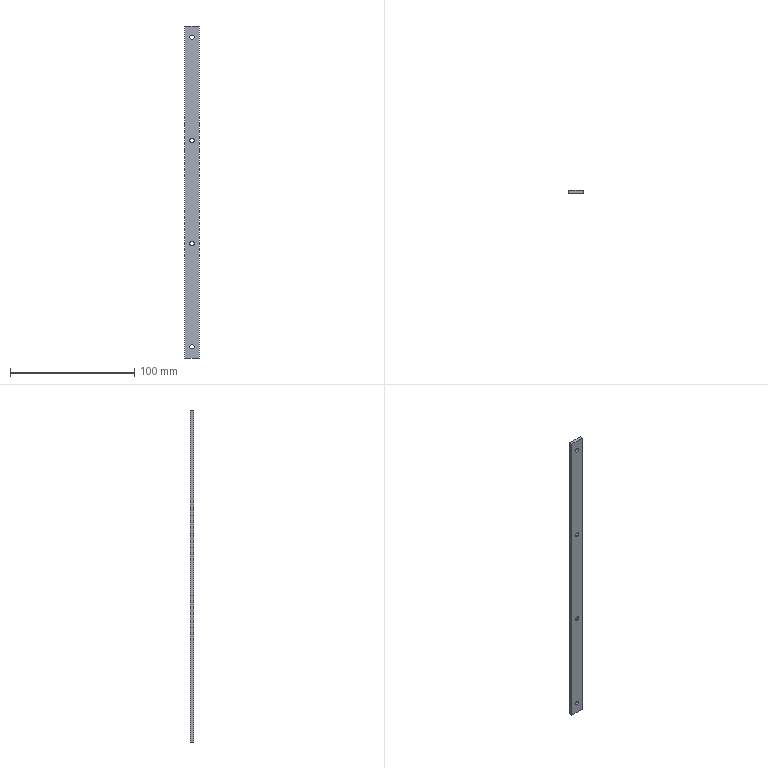Part | NX | features solid 2 | 1 solid | 14 faces | box 12 x 2.5 x 267 mm | volume 7916 mm3 | cylinder 8 | plane 6 | commonest cylinder face diameters 3.459 x8
STEP:
#1=CARTESIAN_POINT('',(339.,-655.,348.229));
#2=VERTEX_POINT('',#1);
#3=CARTESIAN_POINT('',(339.,-657.5,348.229));
#4=VERTEX_POINT('',#3);
#5=CARTESIAN_POINT('',(339.,-922.281,348.229));
#6=DIRECTION('',(0.,1.,0.));
#7=VECTOR('',#6,1000.);
#8=LINE('',#5,#7);
#9=EDGE_CURVE('',#2,#4,#8,.F.);
#10=ORIENTED_EDGE('',*,*,#9,.T.);
#11=CARTESIAN_POINT('',(339.,-657.5,344.77));
#12=VERTEX_POINT('',#11);
#13=CARTESIAN_POINT('',(339.,-657.5,346.5));
#14=DIRECTION('',(0.,1.,0.));
#15=DIRECTION('',(0.,0.,-1.));
#16=AXIS2_PLACEMENT_3D('',#13,#14,#15);
#17=CIRCLE('',#16,1.73);
#18=EDGE_CURVE('',#12,#4,#17,.T.);
#19=ORIENTED_EDGE('',*,*,#18,.F.);
#20=CARTESIAN_POINT('',(339.,-655.,344.77));
#21=VERTEX_POINT('',#20);
#22=CARTESIAN_POINT('',(339.,-922.281,344.77));
#23=DIRECTION('',(0.,1.,0.));
#24=VECTOR('',#23,1000.);
#25=LINE('',#22,#24);
#26=EDGE_CURVE('',#12,#21,#25,.T.);
#27=ORIENTED_EDGE('',*,*,#26,.T.);
#28=CARTESIAN_POINT('',(339.,-655.,346.5));
#29=DIRECTION('',(0.,1.,0.));
#30=DIRECTION('',(0.,0.,-1.));
#31=AXIS2_PLACEMENT_3D('',#28,#29,#30);
#32=CIRCLE('',#31,1.73);
#33=EDGE_CURVE('',#21,#2,#32,.T.);
#34=ORIENTED_EDGE('',*,*,#33,.T.);
#35=EDGE_LOOP('',(#10,#19,#27,#34));
#36=FACE_BOUND('',#35,.T.);
#37=CARTESIAN_POINT('',(339.,-922.281,346.5));
#38=DIRECTION('',(0.,1.,0.));
#39=DIRECTION('',(0.,0.,-1.));
#40=AXIS2_PLACEMENT_3D('',#37,#38,#39);
#41=CYLINDRICAL_SURFACE('',#40,1.73);
#42=ADVANCED_FACE('',(#36),#41,.F.);
#43=CARTESIAN_POINT('',(339.,-657.5,597.229));
#44=VERTEX_POINT('',#43);
#45=CARTESIAN_POINT('',(339.,-655.,597.229));
#46=VERTEX_POINT('',#45);
#47=CARTESIAN_POINT('',(339.,-922.281,597.229));
#48=DIRECTION('',(0.,1.,0.));
#49=VECTOR('',#48,1000.);
#50=LINE('',#47,#49);
#51=EDGE_CURVE('',#44,#46,#50,.T.);
#52=ORIENTED_EDGE('',*,*,#51,.F.);
#53=CARTESIAN_POINT('',(339.,-657.5,593.77));
#54=VERTEX_POINT('',#53);
#55=CARTESIAN_POINT('',(339.,-657.5,595.5));
#56=DIRECTION('',(0.,1.,0.));
#57=DIRECTION('',(0.,0.,-1.));
#58=AXIS2_PLACEMENT_3D('',#55,#56,#57);
#59=CIRCLE('',#58,1.73);
#60=EDGE_CURVE('',#54,#44,#59,.T.);
#61=ORIENTED_EDGE('',*,*,#60,.F.);
#62=CARTESIAN_POINT('',(339.,-655.,593.77));
#63=VERTEX_POINT('',#62);
#64=CARTESIAN_POINT('',(339.,-922.281,593.77));
#65=DIRECTION('',(0.,1.,0.));
#66=VECTOR('',#65,1000.);
#67=LINE('',#64,#66);
#68=EDGE_CURVE('',#63,#54,#67,.F.);
#69=ORIENTED_EDGE('',*,*,#68,.F.);
#70=CARTESIAN_POINT('',(339.,-655.,595.5));
#71=DIRECTION('',(0.,1.,0.));
#72=DIRECTION('',(0.,0.,-1.));
#73=AXIS2_PLACEMENT_3D('',#70,#71,#72);
#74=CIRCLE('',#73,1.73);
#75=EDGE_CURVE('',#63,#46,#74,.T.);
#76=ORIENTED_EDGE('',*,*,#75,.T.);
#77=EDGE_LOOP('',(#52,#61,#69,#76));
#78=FACE_BOUND('',#77,.T.);
#79=CARTESIAN_POINT('',(339.,-922.281,595.5));
#80=DIRECTION('',(0.,1.,0.));
#81=DIRECTION('',(0.,0.,-1.));
#82=AXIS2_PLACEMENT_3D('',#79,#80,#81);
#83=CYLINDRICAL_SURFACE('',#82,1.73);
#84=ADVANCED_FACE('',(#78),#83,.F.);
#85=CARTESIAN_POINT('',(339.,-657.5,431.229));
#86=VERTEX_POINT('',#85);
#87=CARTESIAN_POINT('',(339.,-655.,431.229));
#88=VERTEX_POINT('',#87);
#89=CARTESIAN_POINT('',(339.,-922.281,431.229));
#90=DIRECTION('',(0.,1.,0.));
#91=VECTOR('',#90,1000.);
#92=LINE('',#89,#91);
#93=EDGE_CURVE('',#86,#88,#92,.T.);
#94=ORIENTED_EDGE('',*,*,#93,.F.);
#95=CARTESIAN_POINT('',(339.,-657.5,427.77));
#96=VERTEX_POINT('',#95);
#97=CARTESIAN_POINT('',(339.,-657.5,429.5));
#98=DIRECTION('',(0.,1.,0.));
#99=DIRECTION('',(0.,0.,-1.));
#100=AXIS2_PLACEMENT_3D('',#97,#98,#99);
#101=CIRCLE('',#100,1.73);
#102=EDGE_CURVE('',#96,#86,#101,.T.);
#103=ORIENTED_EDGE('',*,*,#102,.F.);
#104=CARTESIAN_POINT('',(339.,-655.,427.77));
#105=VERTEX_POINT('',#104);
#106=CARTESIAN_POINT('',(339.,-922.281,427.77));
#107=DIRECTION('',(0.,1.,0.));
#108=VECTOR('',#107,1000.);
#109=LINE('',#106,#108);
#110=EDGE_CURVE('',#105,#96,#109,.F.);
#111=ORIENTED_EDGE('',*,*,#110,.F.);
#112=CARTESIAN_POINT('',(339.,-655.,429.5));
#113=DIRECTION('',(0.,1.,0.));
#114=DIRECTION('',(0.,0.,-1.));
#115=AXIS2_PLACEMENT_3D('',#112,#113,#114);
#116=CIRCLE('',#115,1.73);
#117=EDGE_CURVE('',#105,#88,#116,.T.);
#118=ORIENTED_EDGE('',*,*,#117,.T.);
#119=EDGE_LOOP('',(#94,#103,#111,#118));
#120=FACE_BOUND('',#119,.T.);
#121=CARTESIAN_POINT('',(339.,-922.281,429.5));
#122=DIRECTION('',(0.,1.,0.));
#123=DIRECTION('',(0.,0.,-1.));
#124=AXIS2_PLACEMENT_3D('',#121,#122,#123);
#125=CYLINDRICAL_SURFACE('',#124,1.73);
#126=ADVANCED_FACE('',(#120),#125,.F.);
#127=CARTESIAN_POINT('',(339.,-657.5,514.229));
#128=VERTEX_POINT('',#127);
#129=CARTESIAN_POINT('',(339.,-655.,514.229));
#130=VERTEX_POINT('',#129);
#131=CARTESIAN_POINT('',(339.,-922.281,514.229));
#132=DIRECTION('',(0.,1.,0.));
#133=VECTOR('',#132,1000.);
#134=LINE('',#131,#133);
#135=EDGE_CURVE('',#128,#130,#134,.T.);
#136=ORIENTED_EDGE('',*,*,#135,.F.);
#137=CARTESIAN_POINT('',(339.,-657.5,510.77));
#138=VERTEX_POINT('',#137);
#139=CARTESIAN_POINT('',(339.,-657.5,512.5));
#140=DIRECTION('',(0.,1.,0.));
#141=DIRECTION('',(0.,0.,-1.));
#142=AXIS2_PLACEMENT_3D('',#139,#140,#141);
#143=CIRCLE('',#142,1.73);
#144=EDGE_CURVE('',#138,#128,#143,.T.);
#145=ORIENTED_EDGE('',*,*,#144,.F.);
#146=CARTESIAN_POINT('',(339.,-655.,510.77));
#147=VERTEX_POINT('',#146);
#148=CARTESIAN_POINT('',(339.,-922.281,510.77));
#149=DIRECTION('',(0.,1.,0.));
#150=VECTOR('',#149,1000.);
#151=LINE('',#148,#150);
#152=EDGE_CURVE('',#147,#138,#151,.F.);
#153=ORIENTED_EDGE('',*,*,#152,.F.);
#154=CARTESIAN_POINT('',(339.,-655.,512.5));
#155=DIRECTION('',(0.,1.,0.));
#156=DIRECTION('',(0.,0.,-1.));
#157=AXIS2_PLACEMENT_3D('',#154,#155,#156);
#158=CIRCLE('',#157,1.73);
#159=EDGE_CURVE('',#147,#130,#158,.T.);
#160=ORIENTED_EDGE('',*,*,#159,.T.);
#161=EDGE_LOOP('',(#136,#145,#153,#160));
#162=FACE_BOUND('',#161,.T.);
#163=CARTESIAN_POINT('',(339.,-922.281,512.5));
#164=DIRECTION('',(0.,1.,0.));
#165=DIRECTION('',(0.,0.,-1.));
#166=AXIS2_PLACEMENT_3D('',#163,#164,#165);
#167=CYLINDRICAL_SURFACE('',#166,1.73);
#168=ADVANCED_FACE('',(#162),#167,.F.);
#169=ORIENTED_EDGE('',*,*,#159,.F.);
#170=CARTESIAN_POINT('',(339.,-655.,512.5));
#171=DIRECTION('',(0.,1.,0.));
#172=DIRECTION('',(0.,0.,-1.));
#173=AXIS2_PLACEMENT_3D('',#170,#171,#172);
#174=CIRCLE('',#173,1.73);
#175=EDGE_CURVE('',#130,#147,#174,.T.);
#176=ORIENTED_EDGE('',*,*,#175,.F.);
#177=EDGE_LOOP('',(#169,#176));
#178=FACE_BOUND('',#177,.T.);
#179=ORIENTED_EDGE('',*,*,#117,.F.);
#180=CARTESIAN_POINT('',(339.,-655.,429.5));
#181=DIRECTION('',(0.,1.,0.));
#182=DIRECTION('',(0.,0.,-1.));
#183=AXIS2_PLACEMENT_3D('',#180,#181,#182);
#184=CIRCLE('',#183,1.73);
#185=EDGE_CURVE('',#88,#105,#184,.T.);
#186=ORIENTED_EDGE('',*,*,#185,.F.);
#187=EDGE_LOOP('',(#179,#186));
#188=FACE_BOUND('',#187,.T.);
#189=ORIENTED_EDGE('',*,*,#75,.F.);
#190=CARTESIAN_POINT('',(339.,-655.,595.5));
#191=DIRECTION('',(0.,1.,0.));
#192=DIRECTION('',(0.,0.,-1.));
#193=AXIS2_PLACEMENT_3D('',#190,#191,#192);
#194=CIRCLE('',#193,1.73);
#195=EDGE_CURVE('',#46,#63,#194,.T.);
#196=ORIENTED_EDGE('',*,*,#195,.F.);
#197=EDGE_LOOP('',(#189,#196));
#198=FACE_BOUND('',#197,.T.);
#199=ORIENTED_EDGE('',*,*,#33,.F.);
#200=CARTESIAN_POINT('',(339.,-655.,346.5));
#201=DIRECTION('',(0.,1.,0.));
#202=DIRECTION('',(0.,0.,-1.));
#203=AXIS2_PLACEMENT_3D('',#200,#201,#202);
#204=CIRCLE('',#203,1.73);
#205=EDGE_CURVE('',#2,#21,#204,.T.);
#206=ORIENTED_EDGE('',*,*,#205,.F.);
#207=EDGE_LOOP('',(#199,#206));
#208=FACE_BOUND('',#207,.T.);
#209=CARTESIAN_POINT('',(345.,-655.,337.5));
#210=VERTEX_POINT('',#209);
#211=CARTESIAN_POINT('',(333.,-655.,337.5));
#212=VERTEX_POINT('',#211);
#213=CARTESIAN_POINT('',(345.,-655.,337.5));
#214=DIRECTION('',(-1.,0.,0.));
#215=VECTOR('',#214,1000.);
#216=LINE('',#213,#215);
#217=EDGE_CURVE('',#210,#212,#216,.T.);
#218=ORIENTED_EDGE('',*,*,#217,.T.);
#219=CARTESIAN_POINT('',(333.,-655.,604.5));
#220=VERTEX_POINT('',#219);
#221=CARTESIAN_POINT('',(333.,-655.,337.5));
#222=DIRECTION('',(0.,0.,1.));
#223=VECTOR('',#222,1000.);
#224=LINE('',#221,#223);
#225=EDGE_CURVE('',#212,#220,#224,.T.);
#226=ORIENTED_EDGE('',*,*,#225,.T.);
#227=CARTESIAN_POINT('',(345.,-655.,604.5));
#228=VERTEX_POINT('',#227);
#229=CARTESIAN_POINT('',(345.,-655.,604.5));
#230=DIRECTION('',(1.,0.,0.));
#231=VECTOR('',#230,1000.);
#232=LINE('',#229,#231);
#233=EDGE_CURVE('',#220,#228,#232,.T.);
#234=ORIENTED_EDGE('',*,*,#233,.T.);
#235=CARTESIAN_POINT('',(345.,-655.,337.5));
#236=DIRECTION('',(0.,0.,-1.));
#237=VECTOR('',#236,1000.);
#238=LINE('',#235,#237);
#239=EDGE_CURVE('',#228,#210,#238,.T.);
#240=ORIENTED_EDGE('',*,*,#239,.T.);
#241=EDGE_LOOP('',(#218,#226,#234,#240));
#242=FACE_BOUND('',#241,.T.);
#243=CARTESIAN_POINT('',(339.,-655.,471.));
#244=DIRECTION('',(0.,1.,0.));
#245=DIRECTION('',(0.,0.,-1.));
#246=AXIS2_PLACEMENT_3D('',#243,#244,#245);
#247=PLANE('',#246);
#248=ADVANCED_FACE('',(#178,#188,#198,#208,#242),#247,.T.);
#249=ORIENTED_EDGE('',*,*,#144,.T.);
#250=CARTESIAN_POINT('',(339.,-657.5,512.5));
#251=DIRECTION('',(0.,1.,0.));
#252=DIRECTION('',(0.,0.,-1.));
#253=AXIS2_PLACEMENT_3D('',#250,#251,#252);
#254=CIRCLE('',#253,1.73);
#255=EDGE_CURVE('',#128,#138,#254,.T.);
#256=ORIENTED_EDGE('',*,*,#255,.T.);
#257=EDGE_LOOP('',(#249,#256));
#258=FACE_BOUND('',#257,.T.);
#259=ORIENTED_EDGE('',*,*,#102,.T.);
#260=CARTESIAN_POINT('',(339.,-657.5,429.5));
#261=DIRECTION('',(0.,1.,0.));
#262=DIRECTION('',(0.,0.,-1.));
#263=AXIS2_PLACEMENT_3D('',#260,#261,#262);
#264=CIRCLE('',#263,1.73);
#265=EDGE_CURVE('',#86,#96,#264,.T.);
#266=ORIENTED_EDGE('',*,*,#265,.T.);
#267=EDGE_LOOP('',(#259,#266));
#268=FACE_BOUND('',#267,.T.);
#269=ORIENTED_EDGE('',*,*,#60,.T.);
#270=CARTESIAN_POINT('',(339.,-657.5,595.5));
#271=DIRECTION('',(0.,1.,0.));
#272=DIRECTION('',(0.,0.,-1.));
#273=AXIS2_PLACEMENT_3D('',#270,#271,#272);
#274=CIRCLE('',#273,1.73);
#275=EDGE_CURVE('',#44,#54,#274,.T.);
#276=ORIENTED_EDGE('',*,*,#275,.T.);
#277=EDGE_LOOP('',(#269,#276));
#278=FACE_BOUND('',#277,.T.);
#279=ORIENTED_EDGE('',*,*,#18,.T.);
#280=CARTESIAN_POINT('',(339.,-657.5,346.5));
#281=DIRECTION('',(0.,1.,0.));
#282=DIRECTION('',(0.,0.,-1.));
#283=AXIS2_PLACEMENT_3D('',#280,#281,#282);
#284=CIRCLE('',#283,1.73);
#285=EDGE_CURVE('',#4,#12,#284,.T.);
#286=ORIENTED_EDGE('',*,*,#285,.T.);
#287=EDGE_LOOP('',(#279,#286));
#288=FACE_BOUND('',#287,.T.);
#289=CARTESIAN_POINT('',(345.,-657.5,337.5));
#290=VERTEX_POINT('',#289);
#291=CARTESIAN_POINT('',(333.,-657.5,337.5));
#292=VERTEX_POINT('',#291);
#293=CARTESIAN_POINT('',(345.,-657.5,337.5));
#294=DIRECTION('',(-1.,0.,0.));
#295=VECTOR('',#294,1000.);
#296=LINE('',#293,#295);
#297=EDGE_CURVE('',#290,#292,#296,.T.);
#298=ORIENTED_EDGE('',*,*,#297,.F.);
#299=CARTESIAN_POINT('',(345.,-657.5,604.5));
#300=VERTEX_POINT('',#299);
#301=CARTESIAN_POINT('',(345.,-657.5,337.5));
#302=DIRECTION('',(0.,0.,-1.));
#303=VECTOR('',#302,1000.);
#304=LINE('',#301,#303);
#305=EDGE_CURVE('',#300,#290,#304,.T.);
#306=ORIENTED_EDGE('',*,*,#305,.F.);
#307=CARTESIAN_POINT('',(333.,-657.5,604.5));
#308=VERTEX_POINT('',#307);
#309=CARTESIAN_POINT('',(345.,-657.5,604.5));
#310=DIRECTION('',(1.,0.,0.));
#311=VECTOR('',#310,1000.);
#312=LINE('',#309,#311);
#313=EDGE_CURVE('',#308,#300,#312,.T.);
#314=ORIENTED_EDGE('',*,*,#313,.F.);
#315=CARTESIAN_POINT('',(333.,-657.5,337.5));
#316=DIRECTION('',(0.,0.,1.));
#317=VECTOR('',#316,1000.);
#318=LINE('',#315,#317);
#319=EDGE_CURVE('',#292,#308,#318,.T.);
#320=ORIENTED_EDGE('',*,*,#319,.F.);
#321=EDGE_LOOP('',(#298,#306,#314,#320));
#322=FACE_BOUND('',#321,.T.);
#323=CARTESIAN_POINT('',(339.,-657.5,471.));
#324=DIRECTION('',(0.,1.,0.));
#325=DIRECTION('',(0.,0.,-1.));
#326=AXIS2_PLACEMENT_3D('',#323,#324,#325);
#327=PLANE('',#326);
#328=ADVANCED_FACE('',(#258,#268,#278,#288,#322),#327,.F.);
#329=ORIENTED_EDGE('',*,*,#239,.F.);
#330=CARTESIAN_POINT('',(345.,-657.5,604.5));
#331=DIRECTION('',(0.,1.,0.));
#332=VECTOR('',#331,1000.);
#333=LINE('',#330,#332);
#334=EDGE_CURVE('',#300,#228,#333,.T.);
#335=ORIENTED_EDGE('',*,*,#334,.F.);
#336=ORIENTED_EDGE('',*,*,#305,.T.);
#337=CARTESIAN_POINT('',(345.,-657.5,337.5));
#338=DIRECTION('',(0.,1.,0.));
#339=VECTOR('',#338,1000.);
#340=LINE('',#337,#339);
#341=EDGE_CURVE('',#290,#210,#340,.T.);
#342=ORIENTED_EDGE('',*,*,#341,.T.);
#343=EDGE_LOOP('',(#329,#335,#336,#342));
#344=FACE_BOUND('',#343,.T.);
#345=CARTESIAN_POINT('',(345.,-657.5,337.5));
#346=DIRECTION('',(1.,0.,0.));
#347=DIRECTION('',(0.,0.,1.));
#348=AXIS2_PLACEMENT_3D('',#345,#346,#347);
#349=PLANE('',#348);
#350=ADVANCED_FACE('',(#344),#349,.T.);
#351=ORIENTED_EDGE('',*,*,#233,.F.);
#352=CARTESIAN_POINT('',(333.,-657.5,604.5));
#353=DIRECTION('',(0.,1.,0.));
#354=VECTOR('',#353,1000.);
#355=LINE('',#352,#354);
#356=EDGE_CURVE('',#308,#220,#355,.T.);
#357=ORIENTED_EDGE('',*,*,#356,.F.);
#358=ORIENTED_EDGE('',*,*,#313,.T.);
#359=ORIENTED_EDGE('',*,*,#334,.T.);
#360=EDGE_LOOP('',(#351,#357,#358,#359));
#361=FACE_BOUND('',#360,.T.);
#362=CARTESIAN_POINT('',(345.,-657.5,604.5));
#363=DIRECTION('',(0.,0.,1.));
#364=DIRECTION('',(1.,0.,0.));
#365=AXIS2_PLACEMENT_3D('',#362,#363,#364);
#366=PLANE('',#365);
#367=ADVANCED_FACE('',(#361),#366,.T.);
#368=ORIENTED_EDGE('',*,*,#225,.F.);
#369=CARTESIAN_POINT('',(333.,-657.5,337.5));
#370=DIRECTION('',(0.,1.,0.));
#371=VECTOR('',#370,1000.);
#372=LINE('',#369,#371);
#373=EDGE_CURVE('',#292,#212,#372,.T.);
#374=ORIENTED_EDGE('',*,*,#373,.F.);
#375=ORIENTED_EDGE('',*,*,#319,.T.);
#376=ORIENTED_EDGE('',*,*,#356,.T.);
#377=EDGE_LOOP('',(#368,#374,#375,#376));
#378=FACE_BOUND('',#377,.T.);
#379=CARTESIAN_POINT('',(333.,-657.5,337.5));
#380=DIRECTION('',(-1.,0.,0.));
#381=DIRECTION('',(0.,0.,1.));
#382=AXIS2_PLACEMENT_3D('',#379,#380,#381);
#383=PLANE('',#382);
#384=ADVANCED_FACE('',(#378),#383,.T.);
#385=ORIENTED_EDGE('',*,*,#217,.F.);
#386=ORIENTED_EDGE('',*,*,#341,.F.);
#387=ORIENTED_EDGE('',*,*,#297,.T.);
#388=ORIENTED_EDGE('',*,*,#373,.T.);
#389=EDGE_LOOP('',(#385,#386,#387,#388));
#390=FACE_BOUND('',#389,.T.);
#391=CARTESIAN_POINT('',(345.,-657.5,337.5));
#392=DIRECTION('',(0.,0.,-1.));
#393=DIRECTION('',(0.,-1.,0.));
#394=AXIS2_PLACEMENT_3D('',#391,#392,#393);
#395=PLANE('',#394);
#396=ADVANCED_FACE('',(#390),#395,.T.);
#397=ORIENTED_EDGE('',*,*,#255,.F.);
#398=ORIENTED_EDGE('',*,*,#135,.T.);
#399=ORIENTED_EDGE('',*,*,#175,.T.);
#400=ORIENTED_EDGE('',*,*,#152,.T.);
#401=EDGE_LOOP('',(#397,#398,#399,#400));
#402=FACE_BOUND('',#401,.T.);
#403=CARTESIAN_POINT('',(339.,-922.281,512.5));
#404=DIRECTION('',(0.,1.,0.));
#405=DIRECTION('',(0.,0.,-1.));
#406=AXIS2_PLACEMENT_3D('',#403,#404,#405);
#407=CYLINDRICAL_SURFACE('',#406,1.73);
#408=ADVANCED_FACE('',(#402),#407,.F.);
#409=ORIENTED_EDGE('',*,*,#265,.F.);
#410=ORIENTED_EDGE('',*,*,#93,.T.);
#411=ORIENTED_EDGE('',*,*,#185,.T.);
#412=ORIENTED_EDGE('',*,*,#110,.T.);
#413=EDGE_LOOP('',(#409,#410,#411,#412));
#414=FACE_BOUND('',#413,.T.);
#415=CARTESIAN_POINT('',(339.,-922.281,429.5));
#416=DIRECTION('',(0.,1.,0.));
#417=DIRECTION('',(0.,0.,-1.));
#418=AXIS2_PLACEMENT_3D('',#415,#416,#417);
#419=CYLINDRICAL_SURFACE('',#418,1.73);
#420=ADVANCED_FACE('',(#414),#419,.F.);
#421=ORIENTED_EDGE('',*,*,#275,.F.);
#422=ORIENTED_EDGE('',*,*,#51,.T.);
#423=ORIENTED_EDGE('',*,*,#195,.T.);
#424=ORIENTED_EDGE('',*,*,#68,.T.);
#425=EDGE_LOOP('',(#421,#422,#423,#424));
#426=FACE_BOUND('',#425,.T.);
#427=CARTESIAN_POINT('',(339.,-922.281,595.5));
#428=DIRECTION('',(0.,1.,0.));
#429=DIRECTION('',(0.,0.,-1.));
#430=AXIS2_PLACEMENT_3D('',#427,#428,#429);
#431=CYLINDRICAL_SURFACE('',#430,1.73);
#432=ADVANCED_FACE('',(#426),#431,.F.);
#433=ORIENTED_EDGE('',*,*,#285,.F.);
#434=ORIENTED_EDGE('',*,*,#9,.F.);
#435=ORIENTED_EDGE('',*,*,#205,.T.);
#436=ORIENTED_EDGE('',*,*,#26,.F.);
#437=EDGE_LOOP('',(#433,#434,#435,#436));
#438=FACE_BOUND('',#437,.T.);
#439=CARTESIAN_POINT('',(339.,-922.281,346.5));
#440=DIRECTION('',(0.,1.,0.));
#441=DIRECTION('',(0.,0.,-1.));
#442=AXIS2_PLACEMENT_3D('',#439,#440,#441);
#443=CYLINDRICAL_SURFACE('',#442,1.73);
#444=ADVANCED_FACE('',(#438),#443,.F.);
#445=CLOSED_SHELL('',(#42,#84,#126,#168,#248,#328,#350,#367,#384,#396,#408,#420,#432,#444));
#446=MANIFOLD_SOLID_BREP('',#445);
#447=(LENGTH_UNIT()NAMED_UNIT(*)SI_UNIT(.MILLI.,.METRE.));
#448=UNCERTAINTY_MEASURE_WITH_UNIT(LENGTH_MEASURE(0.00001),#447,'','');
#449=(NAMED_UNIT(*)PLANE_ANGLE_UNIT()SI_UNIT($,.RADIAN.));
#450=(NAMED_UNIT(*)SI_UNIT($,.STERADIAN.)SOLID_ANGLE_UNIT());
#451=(GEOMETRIC_REPRESENTATION_CONTEXT(3)GLOBAL_UNCERTAINTY_ASSIGNED_CONTEXT((#448))GLOBAL_UNIT_ASSIGNED_CONTEXT((#447,#449,#450))REPRESENTATION_CONTEXT('',''));
#452=ADVANCED_BREP_SHAPE_REPRESENTATION('',(#446),#451);